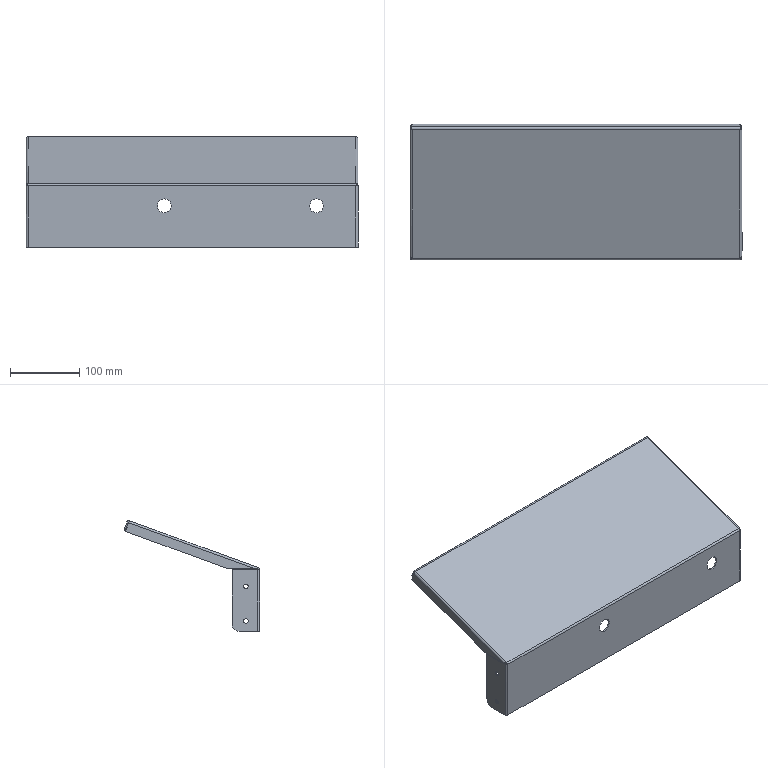Part | SolidWorks | features EdgeFlange 8, ICE 2, Fillet 1, FlatPattern 1, SMBaseFlange 1, SheetMetal 1 | 1 solid | 94 faces | box 480 x 195.932 x 160.122 mm | volume 336686 mm3 | plane 62 | cylinder 30 | spline 2 | commonest cylinder face diameters 2 x8 6 x8 6.5 x8 20 x6